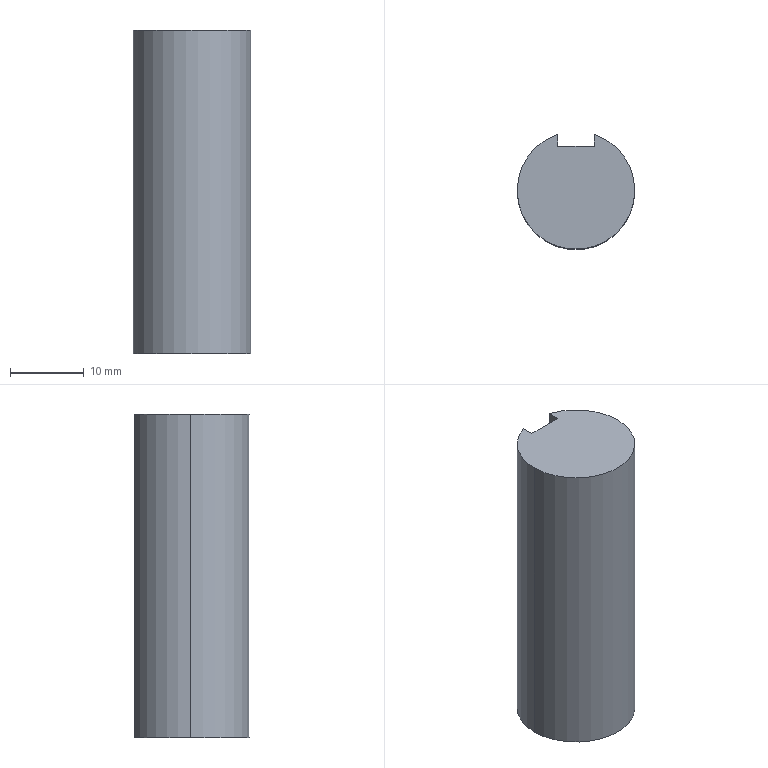Part | SolidWorks | features Extrusion 1 | 1 solid | 8 faces | box 16 x 15.599 x 44 mm | volume 8436 mm3 | plane 5 | cylinder 3 | commonest cylinder face diameters 16 x3
STEP:
#1=CARTESIAN_POINT('',(-276.5,7.599,-44.));
#2=VERTEX_POINT('',#1);
#3=CARTESIAN_POINT('',(-282.,0.,-44.));
#4=VERTEX_POINT('',#3);
#5=CARTESIAN_POINT('',(-274.,0.,-44.));
#6=DIRECTION('',(0.,0.,1.));
#7=DIRECTION('',(-1.,0.,0.));
#8=AXIS2_PLACEMENT_3D('',#5,#6,#7);
#9=CIRCLE('',#8,8.);
#10=EDGE_CURVE('',#2,#4,#9,.T.);
#11=ORIENTED_EDGE('',*,*,#10,.T.);
#12=CARTESIAN_POINT('',(-282.,0.,0.));
#13=VERTEX_POINT('',#12);
#14=CARTESIAN_POINT('',(-282.,0.,-66.346));
#15=DIRECTION('',(0.,0.,1.));
#16=VECTOR('',#15,1000.);
#17=LINE('',#14,#16);
#18=EDGE_CURVE('',#4,#13,#17,.T.);
#19=ORIENTED_EDGE('',*,*,#18,.T.);
#20=CARTESIAN_POINT('',(-276.5,7.599,0.));
#21=VERTEX_POINT('',#20);
#22=CARTESIAN_POINT('',(-274.,0.,0.));
#23=DIRECTION('',(0.,0.,1.));
#24=DIRECTION('',(1.,0.,0.));
#25=AXIS2_PLACEMENT_3D('',#22,#23,#24);
#26=CIRCLE('',#25,8.);
#27=EDGE_CURVE('',#21,#13,#26,.T.);
#28=ORIENTED_EDGE('',*,*,#27,.F.);
#29=CARTESIAN_POINT('',(-276.5,7.599,-66.346));
#30=DIRECTION('',(0.,0.,1.));
#31=VECTOR('',#30,1000.);
#32=LINE('',#29,#31);
#33=EDGE_CURVE('',#2,#21,#32,.T.);
#34=ORIENTED_EDGE('',*,*,#33,.F.);
#35=EDGE_LOOP('',(#11,#19,#28,#34));
#36=FACE_OUTER_BOUND('',#35,.T.);
#37=CARTESIAN_POINT('',(-274.,0.,-66.346));
#38=DIRECTION('',(0.,0.,1.));
#39=DIRECTION('',(1.,0.,0.));
#40=AXIS2_PLACEMENT_3D('',#37,#38,#39);
#41=CYLINDRICAL_SURFACE('',#40,8.);
#42=ADVANCED_FACE('',(#36),#41,.T.);
#43=ORIENTED_EDGE('',*,*,#18,.F.);
#44=CARTESIAN_POINT('',(-266.,0.,-44.));
#45=VERTEX_POINT('',#44);
#46=CARTESIAN_POINT('',(-274.,0.,-44.));
#47=DIRECTION('',(0.,0.,1.));
#48=DIRECTION('',(-1.,0.,0.));
#49=AXIS2_PLACEMENT_3D('',#46,#47,#48);
#50=CIRCLE('',#49,8.);
#51=EDGE_CURVE('',#4,#45,#50,.T.);
#52=ORIENTED_EDGE('',*,*,#51,.T.);
#53=CARTESIAN_POINT('',(-266.,0.,0.));
#54=VERTEX_POINT('',#53);
#55=CARTESIAN_POINT('',(-266.,0.,-66.346));
#56=DIRECTION('',(0.,0.,1.));
#57=VECTOR('',#56,1000.);
#58=LINE('',#55,#57);
#59=EDGE_CURVE('',#45,#54,#58,.T.);
#60=ORIENTED_EDGE('',*,*,#59,.T.);
#61=CARTESIAN_POINT('',(-274.,0.,0.));
#62=DIRECTION('',(0.,0.,1.));
#63=DIRECTION('',(1.,0.,0.));
#64=AXIS2_PLACEMENT_3D('',#61,#62,#63);
#65=CIRCLE('',#64,8.);
#66=EDGE_CURVE('',#13,#54,#65,.T.);
#67=ORIENTED_EDGE('',*,*,#66,.F.);
#68=EDGE_LOOP('',(#43,#52,#60,#67));
#69=FACE_OUTER_BOUND('',#68,.T.);
#70=CARTESIAN_POINT('',(-274.,0.,-66.346));
#71=DIRECTION('',(0.,0.,1.));
#72=DIRECTION('',(1.,0.,0.));
#73=AXIS2_PLACEMENT_3D('',#70,#71,#72);
#74=CYLINDRICAL_SURFACE('',#73,8.);
#75=ADVANCED_FACE('',(#69),#74,.T.);
#76=ORIENTED_EDGE('',*,*,#10,.F.);
#77=CARTESIAN_POINT('',(-276.5,6.,-44.));
#78=VERTEX_POINT('',#77);
#79=CARTESIAN_POINT('',(-276.5,6.,-44.));
#80=DIRECTION('',(0.,1.,0.));
#81=VECTOR('',#80,1000.);
#82=LINE('',#79,#81);
#83=EDGE_CURVE('',#78,#2,#82,.T.);
#84=ORIENTED_EDGE('',*,*,#83,.F.);
#85=CARTESIAN_POINT('',(-271.5,6.,-44.));
#86=VERTEX_POINT('',#85);
#87=CARTESIAN_POINT('',(-271.5,6.,-44.));
#88=DIRECTION('',(-1.,0.,0.));
#89=VECTOR('',#88,1000.);
#90=LINE('',#87,#89);
#91=EDGE_CURVE('',#86,#78,#90,.T.);
#92=ORIENTED_EDGE('',*,*,#91,.F.);
#93=CARTESIAN_POINT('',(-271.5,7.599,-44.));
#94=VERTEX_POINT('',#93);
#95=CARTESIAN_POINT('',(-271.5,6.,-44.));
#96=DIRECTION('',(0.,-1.,0.));
#97=VECTOR('',#96,1000.);
#98=LINE('',#95,#97);
#99=EDGE_CURVE('',#94,#86,#98,.T.);
#100=ORIENTED_EDGE('',*,*,#99,.F.);
#101=CARTESIAN_POINT('',(-274.,0.,-44.));
#102=DIRECTION('',(0.,0.,1.));
#103=DIRECTION('',(-1.,0.,0.));
#104=AXIS2_PLACEMENT_3D('',#101,#102,#103);
#105=CIRCLE('',#104,8.);
#106=EDGE_CURVE('',#45,#94,#105,.T.);
#107=ORIENTED_EDGE('',*,*,#106,.F.);
#108=ORIENTED_EDGE('',*,*,#51,.F.);
#109=EDGE_LOOP('',(#76,#84,#92,#100,#107,#108));
#110=FACE_OUTER_BOUND('',#109,.T.);
#111=CARTESIAN_POINT('',(-274.,17.5,-44.));
#112=DIRECTION('',(0.,0.,-1.));
#113=DIRECTION('',(-1.,0.,0.));
#114=AXIS2_PLACEMENT_3D('',#111,#112,#113);
#115=PLANE('',#114);
#116=ADVANCED_FACE('',(#110),#115,.T.);
#117=ORIENTED_EDGE('',*,*,#27,.T.);
#118=ORIENTED_EDGE('',*,*,#66,.T.);
#119=CARTESIAN_POINT('',(-271.5,7.599,0.));
#120=VERTEX_POINT('',#119);
#121=CARTESIAN_POINT('',(-274.,0.,0.));
#122=DIRECTION('',(0.,0.,1.));
#123=DIRECTION('',(1.,0.,0.));
#124=AXIS2_PLACEMENT_3D('',#121,#122,#123);
#125=CIRCLE('',#124,8.);
#126=EDGE_CURVE('',#54,#120,#125,.T.);
#127=ORIENTED_EDGE('',*,*,#126,.T.);
#128=CARTESIAN_POINT('',(-271.5,6.,0.));
#129=VERTEX_POINT('',#128);
#130=CARTESIAN_POINT('',(-271.5,6.,0.));
#131=DIRECTION('',(0.,-1.,0.));
#132=VECTOR('',#131,1000.);
#133=LINE('',#130,#132);
#134=EDGE_CURVE('',#120,#129,#133,.T.);
#135=ORIENTED_EDGE('',*,*,#134,.T.);
#136=CARTESIAN_POINT('',(-276.5,6.,0.));
#137=VERTEX_POINT('',#136);
#138=CARTESIAN_POINT('',(-271.5,6.,0.));
#139=DIRECTION('',(-1.,0.,0.));
#140=VECTOR('',#139,1000.);
#141=LINE('',#138,#140);
#142=EDGE_CURVE('',#129,#137,#141,.T.);
#143=ORIENTED_EDGE('',*,*,#142,.T.);
#144=CARTESIAN_POINT('',(-276.5,6.,0.));
#145=DIRECTION('',(0.,1.,0.));
#146=VECTOR('',#145,1000.);
#147=LINE('',#144,#146);
#148=EDGE_CURVE('',#137,#21,#147,.T.);
#149=ORIENTED_EDGE('',*,*,#148,.T.);
#150=EDGE_LOOP('',(#117,#118,#127,#135,#143,#149));
#151=FACE_OUTER_BOUND('',#150,.T.);
#152=CARTESIAN_POINT('',(-274.,0.,0.));
#153=DIRECTION('',(0.,0.,1.));
#154=DIRECTION('',(1.,0.,0.));
#155=AXIS2_PLACEMENT_3D('',#152,#153,#154);
#156=PLANE('',#155);
#157=ADVANCED_FACE('',(#151),#156,.T.);
#158=CARTESIAN_POINT('',(-271.5,7.599,-66.346));
#159=DIRECTION('',(0.,0.,1.));
#160=VECTOR('',#159,1000.);
#161=LINE('',#158,#160);
#162=EDGE_CURVE('',#94,#120,#161,.T.);
#163=ORIENTED_EDGE('',*,*,#162,.F.);
#164=ORIENTED_EDGE('',*,*,#99,.T.);
#165=CARTESIAN_POINT('',(-271.5,6.,-66.346));
#166=DIRECTION('',(0.,0.,1.));
#167=VECTOR('',#166,1000.);
#168=LINE('',#165,#167);
#169=EDGE_CURVE('',#86,#129,#168,.T.);
#170=ORIENTED_EDGE('',*,*,#169,.T.);
#171=ORIENTED_EDGE('',*,*,#134,.F.);
#172=EDGE_LOOP('',(#163,#164,#170,#171));
#173=FACE_OUTER_BOUND('',#172,.T.);
#174=CARTESIAN_POINT('',(-271.5,6.,-66.346));
#175=DIRECTION('',(-1.,0.,0.));
#176=DIRECTION('',(0.,0.,1.));
#177=AXIS2_PLACEMENT_3D('',#174,#175,#176);
#178=PLANE('',#177);
#179=ADVANCED_FACE('',(#173),#178,.T.);
#180=ORIENTED_EDGE('',*,*,#169,.F.);
#181=ORIENTED_EDGE('',*,*,#91,.T.);
#182=CARTESIAN_POINT('',(-276.5,6.,-66.346));
#183=DIRECTION('',(0.,0.,1.));
#184=VECTOR('',#183,1000.);
#185=LINE('',#182,#184);
#186=EDGE_CURVE('',#78,#137,#185,.T.);
#187=ORIENTED_EDGE('',*,*,#186,.T.);
#188=ORIENTED_EDGE('',*,*,#142,.F.);
#189=EDGE_LOOP('',(#180,#181,#187,#188));
#190=FACE_OUTER_BOUND('',#189,.T.);
#191=CARTESIAN_POINT('',(-271.5,6.,-66.346));
#192=DIRECTION('',(0.,1.,0.));
#193=DIRECTION('',(0.,0.,1.));
#194=AXIS2_PLACEMENT_3D('',#191,#192,#193);
#195=PLANE('',#194);
#196=ADVANCED_FACE('',(#190),#195,.T.);
#197=ORIENTED_EDGE('',*,*,#186,.F.);
#198=ORIENTED_EDGE('',*,*,#83,.T.);
#199=ORIENTED_EDGE('',*,*,#33,.T.);
#200=ORIENTED_EDGE('',*,*,#148,.F.);
#201=EDGE_LOOP('',(#197,#198,#199,#200));
#202=FACE_OUTER_BOUND('',#201,.T.);
#203=CARTESIAN_POINT('',(-276.5,6.,-66.346));
#204=DIRECTION('',(1.,0.,0.));
#205=DIRECTION('',(0.,0.,-1.));
#206=AXIS2_PLACEMENT_3D('',#203,#204,#205);
#207=PLANE('',#206);
#208=ADVANCED_FACE('',(#202),#207,.T.);
#209=ORIENTED_EDGE('',*,*,#59,.F.);
#210=ORIENTED_EDGE('',*,*,#106,.T.);
#211=ORIENTED_EDGE('',*,*,#162,.T.);
#212=ORIENTED_EDGE('',*,*,#126,.F.);
#213=EDGE_LOOP('',(#209,#210,#211,#212));
#214=FACE_OUTER_BOUND('',#213,.T.);
#215=CARTESIAN_POINT('',(-274.,0.,-66.346));
#216=DIRECTION('',(0.,0.,1.));
#217=DIRECTION('',(1.,0.,0.));
#218=AXIS2_PLACEMENT_3D('',#215,#216,#217);
#219=CYLINDRICAL_SURFACE('',#218,8.);
#220=ADVANCED_FACE('',(#214),#219,.T.);
#221=CLOSED_SHELL('',(#42,#75,#116,#157,#179,#196,#208,#220));
#222=MANIFOLD_SOLID_BREP('',#221);
#223=CARTESIAN_POINT('',(0.,0.,0.));
#224=DIRECTION('',(0.,0.,1.));
#225=DIRECTION('',(1.,0.,0.));
#226=AXIS2_PLACEMENT_3D('',#223,#224,#225);
#227=(LENGTH_UNIT()NAMED_UNIT(*)SI_UNIT(.MILLI.,.METRE.));
#228=UNCERTAINTY_MEASURE_WITH_UNIT(LENGTH_MEASURE(0.00001),#227,'','');
#229=(NAMED_UNIT(*)PLANE_ANGLE_UNIT()SI_UNIT($,.RADIAN.));
#230=(NAMED_UNIT(*)SI_UNIT($,.STERADIAN.)SOLID_ANGLE_UNIT());
#231=(GEOMETRIC_REPRESENTATION_CONTEXT(3)GLOBAL_UNCERTAINTY_ASSIGNED_CONTEXT((#228))GLOBAL_UNIT_ASSIGNED_CONTEXT((#227,#229,#230))REPRESENTATION_CONTEXT('',''));
#232=ADVANCED_BREP_SHAPE_REPRESENTATION('',(#222,#226),#231);